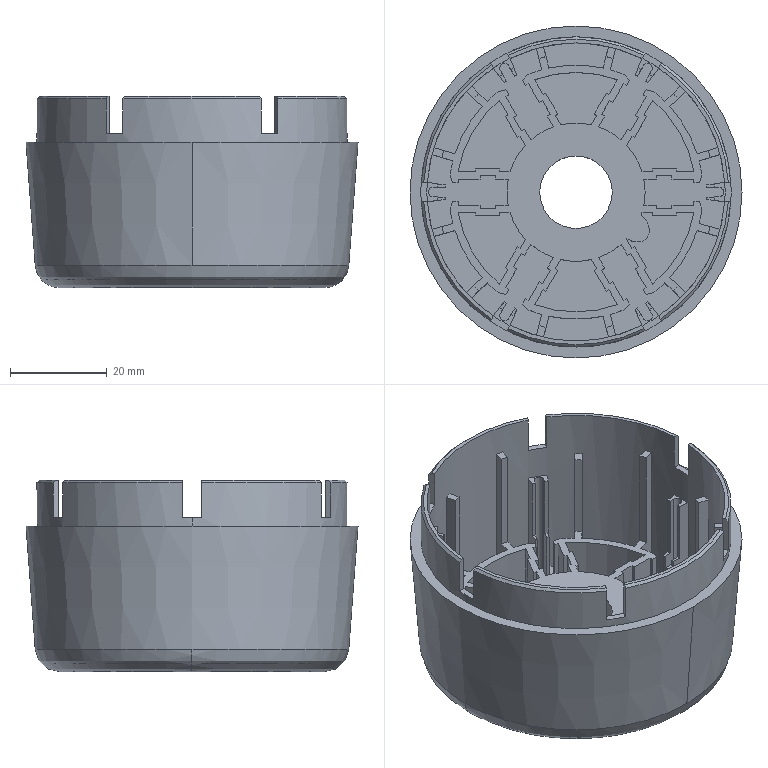Part | STEP file | B01-_X2_70B980F6_X0_ | 1 solid | 380 faces | box 68.5 x 68.5 x 39.5 mm | volume 31380 mm3 | plane 291 | cylinder 77 | cone 8 | torus 2 | spline 2 | commonest cylinder face diameters 57.19 x24 52.4 x18 28.5 x14 2 x9 49.4 x6 15 x2